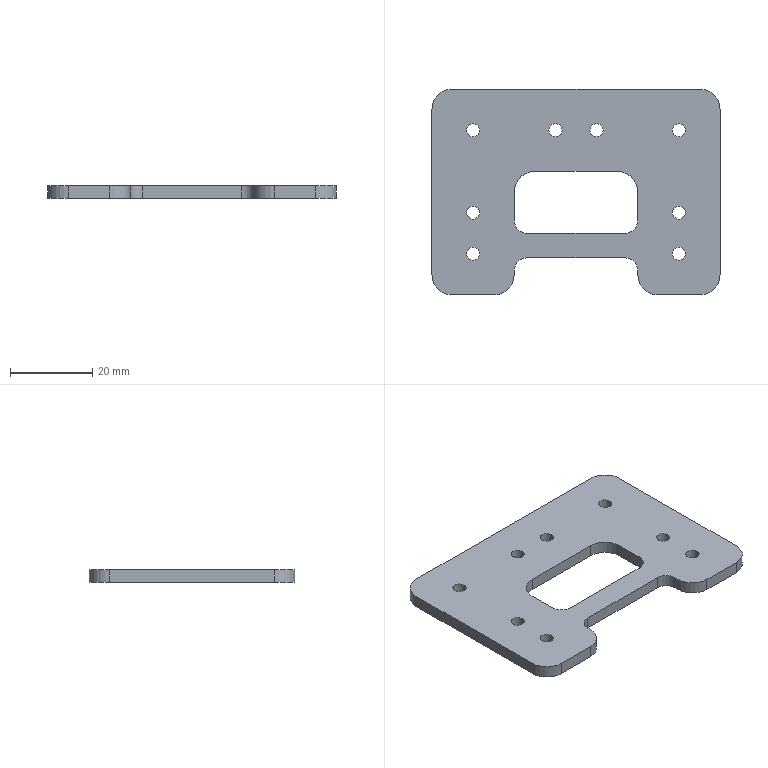Part | SolidWorks | features BaseBody 1 | 1 solid | 42 faces | box 70 x 50 x 3 mm | volume 8106 mm3 | cylinder 28 | plane 14 | commonest cylinder face diameters 3.2 x16 10 x8 6 x4
STEP:
#1=CARTESIAN_POINT('',(26.6,-15.,3.));
#2=VERTEX_POINT('',#1);
#3=CARTESIAN_POINT('',(23.4,-15.,3.));
#4=VERTEX_POINT('',#3);
#5=CARTESIAN_POINT('',(25.,-15.,3.));
#6=DIRECTION('',(0.,0.,-1.));
#7=DIRECTION('',(-1.,0.,0.));
#8=AXIS2_PLACEMENT_3D('',#5,#6,#7);
#9=CIRCLE('',#8,1.6);
#10=EDGE_CURVE('',#2,#4,#9,.T.);
#11=ORIENTED_EDGE('',*,*,#10,.F.);
#12=CARTESIAN_POINT('',(26.6,-15.,0.));
#13=VERTEX_POINT('',#12);
#14=CARTESIAN_POINT('',(26.6,-15.,3.));
#15=DIRECTION('',(0.,0.,-1.));
#16=VECTOR('',#15,1000.);
#17=LINE('',#14,#16);
#18=EDGE_CURVE('',#2,#13,#17,.T.);
#19=ORIENTED_EDGE('',*,*,#18,.T.);
#20=CARTESIAN_POINT('',(23.4,-15.,0.));
#21=VERTEX_POINT('',#20);
#22=CARTESIAN_POINT('',(25.,-15.,0.));
#23=DIRECTION('',(0.,0.,-1.));
#24=DIRECTION('',(-1.,0.,0.));
#25=AXIS2_PLACEMENT_3D('',#22,#23,#24);
#26=CIRCLE('',#25,1.6);
#27=EDGE_CURVE('',#13,#21,#26,.T.);
#28=ORIENTED_EDGE('',*,*,#27,.T.);
#29=CARTESIAN_POINT('',(23.4,-15.,3.));
#30=DIRECTION('',(0.,0.,-1.));
#31=VECTOR('',#30,1000.);
#32=LINE('',#29,#31);
#33=EDGE_CURVE('',#4,#21,#32,.T.);
#34=ORIENTED_EDGE('',*,*,#33,.F.);
#35=EDGE_LOOP('',(#11,#19,#28,#34));
#36=FACE_OUTER_BOUND('',#35,.T.);
#37=CARTESIAN_POINT('',(25.,-15.,3.));
#38=DIRECTION('',(0.,0.,-1.));
#39=DIRECTION('',(-1.,0.,0.));
#40=AXIS2_PLACEMENT_3D('',#37,#38,#39);
#41=CYLINDRICAL_SURFACE('',#40,1.6);
#42=ADVANCED_FACE('',(#36),#41,.F.);
#43=CARTESIAN_POINT('',(26.6,-5.,3.));
#44=VERTEX_POINT('',#43);
#45=CARTESIAN_POINT('',(23.4,-5.,3.));
#46=VERTEX_POINT('',#45);
#47=CARTESIAN_POINT('',(25.,-5.,3.));
#48=DIRECTION('',(0.,0.,-1.));
#49=DIRECTION('',(-1.,0.,0.));
#50=AXIS2_PLACEMENT_3D('',#47,#48,#49);
#51=CIRCLE('',#50,1.6);
#52=EDGE_CURVE('',#44,#46,#51,.T.);
#53=ORIENTED_EDGE('',*,*,#52,.F.);
#54=CARTESIAN_POINT('',(26.6,-5.,0.));
#55=VERTEX_POINT('',#54);
#56=CARTESIAN_POINT('',(26.6,-5.,3.));
#57=DIRECTION('',(0.,0.,-1.));
#58=VECTOR('',#57,1000.);
#59=LINE('',#56,#58);
#60=EDGE_CURVE('',#44,#55,#59,.T.);
#61=ORIENTED_EDGE('',*,*,#60,.T.);
#62=CARTESIAN_POINT('',(23.4,-5.,0.));
#63=VERTEX_POINT('',#62);
#64=CARTESIAN_POINT('',(25.,-5.,0.));
#65=DIRECTION('',(0.,0.,-1.));
#66=DIRECTION('',(-1.,0.,0.));
#67=AXIS2_PLACEMENT_3D('',#64,#65,#66);
#68=CIRCLE('',#67,1.6);
#69=EDGE_CURVE('',#55,#63,#68,.T.);
#70=ORIENTED_EDGE('',*,*,#69,.T.);
#71=CARTESIAN_POINT('',(23.4,-5.,3.));
#72=DIRECTION('',(0.,0.,-1.));
#73=VECTOR('',#72,1000.);
#74=LINE('',#71,#73);
#75=EDGE_CURVE('',#46,#63,#74,.T.);
#76=ORIENTED_EDGE('',*,*,#75,.F.);
#77=EDGE_LOOP('',(#53,#61,#70,#76));
#78=FACE_OUTER_BOUND('',#77,.T.);
#79=CARTESIAN_POINT('',(25.,-5.,3.));
#80=DIRECTION('',(0.,0.,-1.));
#81=DIRECTION('',(-1.,0.,0.));
#82=AXIS2_PLACEMENT_3D('',#79,#80,#81);
#83=CYLINDRICAL_SURFACE('',#82,1.6);
#84=ADVANCED_FACE('',(#78),#83,.F.);
#85=CARTESIAN_POINT('',(26.6,15.,3.));
#86=VERTEX_POINT('',#85);
#87=CARTESIAN_POINT('',(23.4,15.,3.));
#88=VERTEX_POINT('',#87);
#89=CARTESIAN_POINT('',(25.,15.,3.));
#90=DIRECTION('',(0.,0.,-1.));
#91=DIRECTION('',(-1.,0.,0.));
#92=AXIS2_PLACEMENT_3D('',#89,#90,#91);
#93=CIRCLE('',#92,1.6);
#94=EDGE_CURVE('',#86,#88,#93,.T.);
#95=ORIENTED_EDGE('',*,*,#94,.F.);
#96=CARTESIAN_POINT('',(26.6,15.,0.));
#97=VERTEX_POINT('',#96);
#98=CARTESIAN_POINT('',(26.6,15.,3.));
#99=DIRECTION('',(0.,0.,-1.));
#100=VECTOR('',#99,1000.);
#101=LINE('',#98,#100);
#102=EDGE_CURVE('',#86,#97,#101,.T.);
#103=ORIENTED_EDGE('',*,*,#102,.T.);
#104=CARTESIAN_POINT('',(23.4,15.,0.));
#105=VERTEX_POINT('',#104);
#106=CARTESIAN_POINT('',(25.,15.,0.));
#107=DIRECTION('',(0.,0.,-1.));
#108=DIRECTION('',(-1.,0.,0.));
#109=AXIS2_PLACEMENT_3D('',#106,#107,#108);
#110=CIRCLE('',#109,1.6);
#111=EDGE_CURVE('',#97,#105,#110,.T.);
#112=ORIENTED_EDGE('',*,*,#111,.T.);
#113=CARTESIAN_POINT('',(23.4,15.,3.));
#114=DIRECTION('',(0.,0.,-1.));
#115=VECTOR('',#114,1000.);
#116=LINE('',#113,#115);
#117=EDGE_CURVE('',#88,#105,#116,.T.);
#118=ORIENTED_EDGE('',*,*,#117,.F.);
#119=EDGE_LOOP('',(#95,#103,#112,#118));
#120=FACE_OUTER_BOUND('',#119,.T.);
#121=CARTESIAN_POINT('',(25.,15.,3.));
#122=DIRECTION('',(0.,0.,-1.));
#123=DIRECTION('',(-1.,0.,0.));
#124=AXIS2_PLACEMENT_3D('',#121,#122,#123);
#125=CYLINDRICAL_SURFACE('',#124,1.6);
#126=ADVANCED_FACE('',(#120),#125,.F.);
#127=CARTESIAN_POINT('',(6.6,15.,3.));
#128=VERTEX_POINT('',#127);
#129=CARTESIAN_POINT('',(3.4,15.,3.));
#130=VERTEX_POINT('',#129);
#131=CARTESIAN_POINT('',(5.,15.,3.));
#132=DIRECTION('',(0.,0.,-1.));
#133=DIRECTION('',(-1.,0.,0.));
#134=AXIS2_PLACEMENT_3D('',#131,#132,#133);
#135=CIRCLE('',#134,1.6);
#136=EDGE_CURVE('',#128,#130,#135,.T.);
#137=ORIENTED_EDGE('',*,*,#136,.F.);
#138=CARTESIAN_POINT('',(6.6,15.,0.));
#139=VERTEX_POINT('',#138);
#140=CARTESIAN_POINT('',(6.6,15.,3.));
#141=DIRECTION('',(0.,0.,-1.));
#142=VECTOR('',#141,1000.);
#143=LINE('',#140,#142);
#144=EDGE_CURVE('',#128,#139,#143,.T.);
#145=ORIENTED_EDGE('',*,*,#144,.T.);
#146=CARTESIAN_POINT('',(3.4,15.,0.));
#147=VERTEX_POINT('',#146);
#148=CARTESIAN_POINT('',(5.,15.,0.));
#149=DIRECTION('',(0.,0.,-1.));
#150=DIRECTION('',(-1.,0.,0.));
#151=AXIS2_PLACEMENT_3D('',#148,#149,#150);
#152=CIRCLE('',#151,1.6);
#153=EDGE_CURVE('',#139,#147,#152,.T.);
#154=ORIENTED_EDGE('',*,*,#153,.T.);
#155=CARTESIAN_POINT('',(3.4,15.,3.));
#156=DIRECTION('',(0.,0.,-1.));
#157=VECTOR('',#156,1000.);
#158=LINE('',#155,#157);
#159=EDGE_CURVE('',#130,#147,#158,.T.);
#160=ORIENTED_EDGE('',*,*,#159,.F.);
#161=EDGE_LOOP('',(#137,#145,#154,#160));
#162=FACE_OUTER_BOUND('',#161,.T.);
#163=CARTESIAN_POINT('',(5.,15.,3.));
#164=DIRECTION('',(0.,0.,-1.));
#165=DIRECTION('',(-1.,0.,0.));
#166=AXIS2_PLACEMENT_3D('',#163,#164,#165);
#167=CYLINDRICAL_SURFACE('',#166,1.6);
#168=ADVANCED_FACE('',(#162),#167,.F.);
#169=CARTESIAN_POINT('',(-3.4,15.,3.));
#170=VERTEX_POINT('',#169);
#171=CARTESIAN_POINT('',(-6.6,15.,3.));
#172=VERTEX_POINT('',#171);
#173=CARTESIAN_POINT('',(-5.,15.,3.));
#174=DIRECTION('',(0.,0.,-1.));
#175=DIRECTION('',(-1.,0.,0.));
#176=AXIS2_PLACEMENT_3D('',#173,#174,#175);
#177=CIRCLE('',#176,1.6);
#178=EDGE_CURVE('',#170,#172,#177,.T.);
#179=ORIENTED_EDGE('',*,*,#178,.F.);
#180=CARTESIAN_POINT('',(-3.4,15.,0.));
#181=VERTEX_POINT('',#180);
#182=CARTESIAN_POINT('',(-3.4,15.,3.));
#183=DIRECTION('',(0.,0.,-1.));
#184=VECTOR('',#183,1000.);
#185=LINE('',#182,#184);
#186=EDGE_CURVE('',#170,#181,#185,.T.);
#187=ORIENTED_EDGE('',*,*,#186,.T.);
#188=CARTESIAN_POINT('',(-6.6,15.,0.));
#189=VERTEX_POINT('',#188);
#190=CARTESIAN_POINT('',(-5.,15.,0.));
#191=DIRECTION('',(0.,0.,-1.));
#192=DIRECTION('',(-1.,0.,0.));
#193=AXIS2_PLACEMENT_3D('',#190,#191,#192);
#194=CIRCLE('',#193,1.6);
#195=EDGE_CURVE('',#181,#189,#194,.T.);
#196=ORIENTED_EDGE('',*,*,#195,.T.);
#197=CARTESIAN_POINT('',(-6.6,15.,3.));
#198=DIRECTION('',(0.,0.,-1.));
#199=VECTOR('',#198,1000.);
#200=LINE('',#197,#199);
#201=EDGE_CURVE('',#172,#189,#200,.T.);
#202=ORIENTED_EDGE('',*,*,#201,.F.);
#203=EDGE_LOOP('',(#179,#187,#196,#202));
#204=FACE_OUTER_BOUND('',#203,.T.);
#205=CARTESIAN_POINT('',(-5.,15.,3.));
#206=DIRECTION('',(0.,0.,-1.));
#207=DIRECTION('',(-1.,0.,0.));
#208=AXIS2_PLACEMENT_3D('',#205,#206,#207);
#209=CYLINDRICAL_SURFACE('',#208,1.6);
#210=ADVANCED_FACE('',(#204),#209,.F.);
#211=CARTESIAN_POINT('',(-23.4,15.,3.));
#212=VERTEX_POINT('',#211);
#213=CARTESIAN_POINT('',(-26.6,15.,3.));
#214=VERTEX_POINT('',#213);
#215=CARTESIAN_POINT('',(-25.,15.,3.));
#216=DIRECTION('',(0.,0.,-1.));
#217=DIRECTION('',(-1.,0.,0.));
#218=AXIS2_PLACEMENT_3D('',#215,#216,#217);
#219=CIRCLE('',#218,1.6);
#220=EDGE_CURVE('',#212,#214,#219,.T.);
#221=ORIENTED_EDGE('',*,*,#220,.F.);
#222=CARTESIAN_POINT('',(-23.4,15.,0.));
#223=VERTEX_POINT('',#222);
#224=CARTESIAN_POINT('',(-23.4,15.,3.));
#225=DIRECTION('',(0.,0.,-1.));
#226=VECTOR('',#225,1000.);
#227=LINE('',#224,#226);
#228=EDGE_CURVE('',#212,#223,#227,.T.);
#229=ORIENTED_EDGE('',*,*,#228,.T.);
#230=CARTESIAN_POINT('',(-26.6,15.,0.));
#231=VERTEX_POINT('',#230);
#232=CARTESIAN_POINT('',(-25.,15.,0.));
#233=DIRECTION('',(0.,0.,-1.));
#234=DIRECTION('',(-1.,0.,0.));
#235=AXIS2_PLACEMENT_3D('',#232,#233,#234);
#236=CIRCLE('',#235,1.6);
#237=EDGE_CURVE('',#223,#231,#236,.T.);
#238=ORIENTED_EDGE('',*,*,#237,.T.);
#239=CARTESIAN_POINT('',(-26.6,15.,3.));
#240=DIRECTION('',(0.,0.,-1.));
#241=VECTOR('',#240,1000.);
#242=LINE('',#239,#241);
#243=EDGE_CURVE('',#214,#231,#242,.T.);
#244=ORIENTED_EDGE('',*,*,#243,.F.);
#245=EDGE_LOOP('',(#221,#229,#238,#244));
#246=FACE_OUTER_BOUND('',#245,.T.);
#247=CARTESIAN_POINT('',(-25.,15.,3.));
#248=DIRECTION('',(0.,0.,-1.));
#249=DIRECTION('',(-1.,0.,0.));
#250=AXIS2_PLACEMENT_3D('',#247,#248,#249);
#251=CYLINDRICAL_SURFACE('',#250,1.6);
#252=ADVANCED_FACE('',(#246),#251,.F.);
#253=CARTESIAN_POINT('',(-23.4,-5.,3.));
#254=VERTEX_POINT('',#253);
#255=CARTESIAN_POINT('',(-26.6,-5.,3.));
#256=VERTEX_POINT('',#255);
#257=CARTESIAN_POINT('',(-25.,-5.,3.));
#258=DIRECTION('',(0.,0.,-1.));
#259=DIRECTION('',(-1.,0.,0.));
#260=AXIS2_PLACEMENT_3D('',#257,#258,#259);
#261=CIRCLE('',#260,1.6);
#262=EDGE_CURVE('',#254,#256,#261,.T.);
#263=ORIENTED_EDGE('',*,*,#262,.F.);
#264=CARTESIAN_POINT('',(-23.4,-5.,0.));
#265=VERTEX_POINT('',#264);
#266=CARTESIAN_POINT('',(-23.4,-5.,3.));
#267=DIRECTION('',(0.,0.,-1.));
#268=VECTOR('',#267,1000.);
#269=LINE('',#266,#268);
#270=EDGE_CURVE('',#254,#265,#269,.T.);
#271=ORIENTED_EDGE('',*,*,#270,.T.);
#272=CARTESIAN_POINT('',(-26.6,-5.,0.));
#273=VERTEX_POINT('',#272);
#274=CARTESIAN_POINT('',(-25.,-5.,0.));
#275=DIRECTION('',(0.,0.,-1.));
#276=DIRECTION('',(-1.,0.,0.));
#277=AXIS2_PLACEMENT_3D('',#274,#275,#276);
#278=CIRCLE('',#277,1.6);
#279=EDGE_CURVE('',#265,#273,#278,.T.);
#280=ORIENTED_EDGE('',*,*,#279,.T.);
#281=CARTESIAN_POINT('',(-26.6,-5.,3.));
#282=DIRECTION('',(0.,0.,-1.));
#283=VECTOR('',#282,1000.);
#284=LINE('',#281,#283);
#285=EDGE_CURVE('',#256,#273,#284,.T.);
#286=ORIENTED_EDGE('',*,*,#285,.F.);
#287=EDGE_LOOP('',(#263,#271,#280,#286));
#288=FACE_OUTER_BOUND('',#287,.T.);
#289=CARTESIAN_POINT('',(-25.,-5.,3.));
#290=DIRECTION('',(0.,0.,-1.));
#291=DIRECTION('',(-1.,0.,0.));
#292=AXIS2_PLACEMENT_3D('',#289,#290,#291);
#293=CYLINDRICAL_SURFACE('',#292,1.6);
#294=ADVANCED_FACE('',(#288),#293,.F.);
#295=CARTESIAN_POINT('',(-23.4,-15.,3.));
#296=VERTEX_POINT('',#295);
#297=CARTESIAN_POINT('',(-26.6,-15.,3.));
#298=VERTEX_POINT('',#297);
#299=CARTESIAN_POINT('',(-25.,-15.,3.));
#300=DIRECTION('',(0.,0.,-1.));
#301=DIRECTION('',(-1.,0.,0.));
#302=AXIS2_PLACEMENT_3D('',#299,#300,#301);
#303=CIRCLE('',#302,1.6);
#304=EDGE_CURVE('',#296,#298,#303,.T.);
#305=ORIENTED_EDGE('',*,*,#304,.F.);
#306=CARTESIAN_POINT('',(-23.4,-15.,0.));
#307=VERTEX_POINT('',#306);
#308=CARTESIAN_POINT('',(-23.4,-15.,3.));
#309=DIRECTION('',(0.,0.,-1.));
#310=VECTOR('',#309,1000.);
#311=LINE('',#308,#310);
#312=EDGE_CURVE('',#296,#307,#311,.T.);
#313=ORIENTED_EDGE('',*,*,#312,.T.);
#314=CARTESIAN_POINT('',(-26.6,-15.,0.));
#315=VERTEX_POINT('',#314);
#316=CARTESIAN_POINT('',(-25.,-15.,0.));
#317=DIRECTION('',(0.,0.,-1.));
#318=DIRECTION('',(-1.,0.,0.));
#319=AXIS2_PLACEMENT_3D('',#316,#317,#318);
#320=CIRCLE('',#319,1.6);
#321=EDGE_CURVE('',#307,#315,#320,.T.);
#322=ORIENTED_EDGE('',*,*,#321,.T.);
#323=CARTESIAN_POINT('',(-26.6,-15.,3.));
#324=DIRECTION('',(0.,0.,-1.));
#325=VECTOR('',#324,1000.);
#326=LINE('',#323,#325);
#327=EDGE_CURVE('',#298,#315,#326,.T.);
#328=ORIENTED_EDGE('',*,*,#327,.F.);
#329=EDGE_LOOP('',(#305,#313,#322,#328));
#330=FACE_OUTER_BOUND('',#329,.T.);
#331=CARTESIAN_POINT('',(-25.,-15.,3.));
#332=DIRECTION('',(0.,0.,-1.));
#333=DIRECTION('',(-1.,0.,0.));
#334=AXIS2_PLACEMENT_3D('',#331,#332,#333);
#335=CYLINDRICAL_SURFACE('',#334,1.6);
#336=ADVANCED_FACE('',(#330),#335,.F.);
#337=CARTESIAN_POINT('',(25.,-15.,0.));
#338=DIRECTION('',(0.,0.,-1.));
#339=DIRECTION('',(-1.,0.,0.));
#340=AXIS2_PLACEMENT_3D('',#337,#338,#339);
#341=CIRCLE('',#340,1.6);
#342=EDGE_CURVE('',#21,#13,#341,.T.);
#343=ORIENTED_EDGE('',*,*,#342,.F.);
#344=ORIENTED_EDGE('',*,*,#27,.F.);
#345=EDGE_LOOP('',(#343,#344));
#346=FACE_BOUND('',#345,.T.);
#347=CARTESIAN_POINT('',(25.,-5.,0.));
#348=DIRECTION('',(0.,0.,-1.));
#349=DIRECTION('',(-1.,0.,0.));
#350=AXIS2_PLACEMENT_3D('',#347,#348,#349);
#351=CIRCLE('',#350,1.6);
#352=EDGE_CURVE('',#63,#55,#351,.T.);
#353=ORIENTED_EDGE('',*,*,#352,.F.);
#354=ORIENTED_EDGE('',*,*,#69,.F.);
#355=EDGE_LOOP('',(#353,#354));
#356=FACE_BOUND('',#355,.T.);
#357=CARTESIAN_POINT('',(25.,15.,0.));
#358=DIRECTION('',(0.,0.,-1.));
#359=DIRECTION('',(-1.,0.,0.));
#360=AXIS2_PLACEMENT_3D('',#357,#358,#359);
#361=CIRCLE('',#360,1.6);
#362=EDGE_CURVE('',#105,#97,#361,.T.);
#363=ORIENTED_EDGE('',*,*,#362,.F.);
#364=ORIENTED_EDGE('',*,*,#111,.F.);
#365=EDGE_LOOP('',(#363,#364));
#366=FACE_BOUND('',#365,.T.);
#367=CARTESIAN_POINT('',(5.,15.,0.));
#368=DIRECTION('',(0.,0.,-1.));
#369=DIRECTION('',(-1.,0.,0.));
#370=AXIS2_PLACEMENT_3D('',#367,#368,#369);
#371=CIRCLE('',#370,1.6);
#372=EDGE_CURVE('',#147,#139,#371,.T.);
#373=ORIENTED_EDGE('',*,*,#372,.F.);
#374=ORIENTED_EDGE('',*,*,#153,.F.);
#375=EDGE_LOOP('',(#373,#374));
#376=FACE_BOUND('',#375,.T.);
#377=CARTESIAN_POINT('',(-5.,15.,0.));
#378=DIRECTION('',(0.,0.,-1.));
#379=DIRECTION('',(-1.,0.,0.));
#380=AXIS2_PLACEMENT_3D('',#377,#378,#379);
#381=CIRCLE('',#380,1.6);
#382=EDGE_CURVE('',#189,#181,#381,.T.);
#383=ORIENTED_EDGE('',*,*,#382,.F.);
#384=ORIENTED_EDGE('',*,*,#195,.F.);
#385=EDGE_LOOP('',(#383,#384));
#386=FACE_BOUND('',#385,.T.);
#387=CARTESIAN_POINT('',(-25.,15.,0.));
#388=DIRECTION('',(0.,0.,-1.));
#389=DIRECTION('',(-1.,0.,0.));
#390=AXIS2_PLACEMENT_3D('',#387,#388,#389);
#391=CIRCLE('',#390,1.6);
#392=EDGE_CURVE('',#231,#223,#391,.T.);
#393=ORIENTED_EDGE('',*,*,#392,.F.);
#394=ORIENTED_EDGE('',*,*,#237,.F.);
#395=EDGE_LOOP('',(#393,#394));
#396=FACE_BOUND('',#395,.T.);
#397=CARTESIAN_POINT('',(-25.,-5.,0.));
#398=DIRECTION('',(0.,0.,-1.));
#399=DIRECTION('',(-1.,0.,0.));
#400=AXIS2_PLACEMENT_3D('',#397,#398,#399);
#401=CIRCLE('',#400,1.6);
#402=EDGE_CURVE('',#273,#265,#401,.T.);
#403=ORIENTED_EDGE('',*,*,#402,.F.);
#404=ORIENTED_EDGE('',*,*,#279,.F.);
#405=EDGE_LOOP('',(#403,#404));
#406=FACE_BOUND('',#405,.T.);
#407=CARTESIAN_POINT('',(-25.,-15.,0.));
#408=DIRECTION('',(0.,0.,-1.));
#409=DIRECTION('',(-1.,0.,0.));
#410=AXIS2_PLACEMENT_3D('',#407,#408,#409);
#411=CIRCLE('',#410,1.6);
#412=EDGE_CURVE('',#315,#307,#411,.T.);
#413=ORIENTED_EDGE('',*,*,#412,.F.);
#414=ORIENTED_EDGE('',*,*,#321,.F.);
#415=EDGE_LOOP('',(#413,#414));
#416=FACE_BOUND('',#415,.T.);
#417=CARTESIAN_POINT('',(-12.,-10.,0.));
#418=VERTEX_POINT('',#417);
#419=CARTESIAN_POINT('',(-15.,-7.,0.));
#420=VERTEX_POINT('',#419);
#421=CARTESIAN_POINT('',(-12.,-7.,0.));
#422=DIRECTION('',(0.,0.,-1.));
#423=DIRECTION('',(1.,0.,0.));
#424=AXIS2_PLACEMENT_3D('',#421,#422,#423);
#425=CIRCLE('',#424,3.);
#426=EDGE_CURVE('',#418,#420,#425,.T.);
#427=ORIENTED_EDGE('',*,*,#426,.F.);
#428=CARTESIAN_POINT('',(12.,-10.,0.));
#429=VERTEX_POINT('',#428);
#430=CARTESIAN_POINT('',(0.,-10.,0.));
#431=DIRECTION('',(-1.,0.,0.));
#432=VECTOR('',#431,1000.);
#433=LINE('',#430,#432);
#434=EDGE_CURVE('',#429,#418,#433,.T.);
#435=ORIENTED_EDGE('',*,*,#434,.F.);
#436=CARTESIAN_POINT('',(15.,-7.,0.));
#437=VERTEX_POINT('',#436);
#438=CARTESIAN_POINT('',(12.,-7.,0.));
#439=DIRECTION('',(0.,0.,-1.));
#440=DIRECTION('',(1.,0.,0.));
#441=AXIS2_PLACEMENT_3D('',#438,#439,#440);
#442=CIRCLE('',#441,3.);
#443=EDGE_CURVE('',#437,#429,#442,.T.);
#444=ORIENTED_EDGE('',*,*,#443,.F.);
#445=CARTESIAN_POINT('',(15.,0.,0.));
#446=VERTEX_POINT('',#445);
#447=CARTESIAN_POINT('',(15.,0.,0.));
#448=DIRECTION('',(0.,-1.,0.));
#449=VECTOR('',#448,1000.);
#450=LINE('',#447,#449);
#451=EDGE_CURVE('',#446,#437,#450,.T.);
#452=ORIENTED_EDGE('',*,*,#451,.F.);
#453=CARTESIAN_POINT('',(10.,5.,0.));
#454=VERTEX_POINT('',#453);
#455=CARTESIAN_POINT('',(10.,0.,0.));
#456=DIRECTION('',(0.,0.,-1.));
#457=DIRECTION('',(-1.,0.,0.));
#458=AXIS2_PLACEMENT_3D('',#455,#456,#457);
#459=CIRCLE('',#458,5.);
#460=EDGE_CURVE('',#454,#446,#459,.T.);
#461=ORIENTED_EDGE('',*,*,#460,.F.);
#462=CARTESIAN_POINT('',(-10.,5.,0.));
#463=VERTEX_POINT('',#462);
#464=CARTESIAN_POINT('',(0.,5.,0.));
#465=DIRECTION('',(1.,0.,0.));
#466=VECTOR('',#465,1000.);
#467=LINE('',#464,#466);
#468=EDGE_CURVE('',#463,#454,#467,.T.);
#469=ORIENTED_EDGE('',*,*,#468,.F.);
#470=CARTESIAN_POINT('',(-15.,0.,0.));
#471=VERTEX_POINT('',#470);
#472=CARTESIAN_POINT('',(-10.,0.,0.));
#473=DIRECTION('',(0.,0.,-1.));
#474=DIRECTION('',(-1.,0.,0.));
#475=AXIS2_PLACEMENT_3D('',#472,#473,#474);
#476=CIRCLE('',#475,5.);
#477=EDGE_CURVE('',#471,#463,#476,.T.);
#478=ORIENTED_EDGE('',*,*,#477,.F.);
#479=CARTESIAN_POINT('',(-15.,0.,0.));
#480=DIRECTION('',(0.,1.,0.));
#481=VECTOR('',#480,1000.);
#482=LINE('',#479,#481);
#483=EDGE_CURVE('',#420,#471,#482,.T.);
#484=ORIENTED_EDGE('',*,*,#483,.F.);
#485=EDGE_LOOP('',(#427,#435,#444,#452,#461,#469,#478,#484));
#486=FACE_BOUND('',#485,.T.);
#487=CARTESIAN_POINT('',(-15.,-19.,0.));
#488=VERTEX_POINT('',#487);
#489=CARTESIAN_POINT('',(-12.,-16.,0.));
#490=VERTEX_POINT('',#489);
#491=CARTESIAN_POINT('',(-12.,-19.,0.));
#492=DIRECTION('',(0.,0.,-1.));
#493=DIRECTION('',(1.,0.,0.));
#494=AXIS2_PLACEMENT_3D('',#491,#492,#493);
#495=CIRCLE('',#494,3.);
#496=EDGE_CURVE('',#488,#490,#495,.T.);
#497=ORIENTED_EDGE('',*,*,#496,.F.);
#498=CARTESIAN_POINT('',(-15.,-20.,0.));
#499=VERTEX_POINT('',#498);
#500=CARTESIAN_POINT('',(-15.,-25.,0.));
#501=DIRECTION('',(0.,-1.,0.));
#502=VECTOR('',#501,1000.);
#503=LINE('',#500,#502);
#504=EDGE_CURVE('',#488,#499,#503,.T.);
#505=ORIENTED_EDGE('',*,*,#504,.T.);
#506=CARTESIAN_POINT('',(-20.,-25.,0.));
#507=VERTEX_POINT('',#506);
#508=CARTESIAN_POINT('',(-20.,-20.,0.));
#509=DIRECTION('',(0.,0.,1.));
#510=DIRECTION('',(1.,0.,0.));
#511=AXIS2_PLACEMENT_3D('',#508,#509,#510);
#512=CIRCLE('',#511,5.);
#513=EDGE_CURVE('',#507,#499,#512,.T.);
#514=ORIENTED_EDGE('',*,*,#513,.F.);
#515=CARTESIAN_POINT('',(-30.,-25.,0.));
#516=VERTEX_POINT('',#515);
#517=CARTESIAN_POINT('',(0.,-25.,0.));
#518=DIRECTION('',(1.,0.,0.));
#519=VECTOR('',#518,1000.);
#520=LINE('',#517,#519);
#521=EDGE_CURVE('',#516,#507,#520,.T.);
#522=ORIENTED_EDGE('',*,*,#521,.F.);
#523=CARTESIAN_POINT('',(-35.,-20.,0.));
#524=VERTEX_POINT('',#523);
#525=CARTESIAN_POINT('',(-30.,-20.,0.));
#526=DIRECTION('',(0.,0.,1.));
#527=DIRECTION('',(-1.,0.,0.));
#528=AXIS2_PLACEMENT_3D('',#525,#526,#527);
#529=CIRCLE('',#528,5.);
#530=EDGE_CURVE('',#524,#516,#529,.T.);
#531=ORIENTED_EDGE('',*,*,#530,.F.);
#532=CARTESIAN_POINT('',(-35.,20.,0.));
#533=VERTEX_POINT('',#532);
#534=CARTESIAN_POINT('',(-35.,0.,0.));
#535=DIRECTION('',(0.,-1.,0.));
#536=VECTOR('',#535,1000.);
#537=LINE('',#534,#536);
#538=EDGE_CURVE('',#533,#524,#537,.T.);
#539=ORIENTED_EDGE('',*,*,#538,.F.);
#540=CARTESIAN_POINT('',(-30.,25.,0.));
#541=VERTEX_POINT('',#540);
#542=CARTESIAN_POINT('',(-30.,20.,0.));
#543=DIRECTION('',(0.,0.,1.));
#544=DIRECTION('',(-1.,0.,0.));
#545=AXIS2_PLACEMENT_3D('',#542,#543,#544);
#546=CIRCLE('',#545,5.);
#547=EDGE_CURVE('',#541,#533,#546,.T.);
#548=ORIENTED_EDGE('',*,*,#547,.F.);
#549=CARTESIAN_POINT('',(30.,25.,0.));
#550=VERTEX_POINT('',#549);
#551=CARTESIAN_POINT('',(0.,25.,0.));
#552=DIRECTION('',(-1.,0.,0.));
#553=VECTOR('',#552,1000.);
#554=LINE('',#551,#553);
#555=EDGE_CURVE('',#550,#541,#554,.T.);
#556=ORIENTED_EDGE('',*,*,#555,.F.);
#557=CARTESIAN_POINT('',(35.,20.,0.));
#558=VERTEX_POINT('',#557);
#559=CARTESIAN_POINT('',(30.,20.,0.));
#560=DIRECTION('',(0.,0.,1.));
#561=DIRECTION('',(-1.,0.,0.));
#562=AXIS2_PLACEMENT_3D('',#559,#560,#561);
#563=CIRCLE('',#562,5.);
#564=EDGE_CURVE('',#558,#550,#563,.T.);
#565=ORIENTED_EDGE('',*,*,#564,.F.);
#566=CARTESIAN_POINT('',(35.,-20.,0.));
#567=VERTEX_POINT('',#566);
#568=CARTESIAN_POINT('',(35.,0.,0.));
#569=DIRECTION('',(0.,1.,0.));
#570=VECTOR('',#569,1000.);
#571=LINE('',#568,#570);
#572=EDGE_CURVE('',#567,#558,#571,.T.);
#573=ORIENTED_EDGE('',*,*,#572,.F.);
#574=CARTESIAN_POINT('',(30.,-25.,0.));
#575=VERTEX_POINT('',#574);
#576=CARTESIAN_POINT('',(30.,-20.,0.));
#577=DIRECTION('',(0.,0.,1.));
#578=DIRECTION('',(-1.,0.,0.));
#579=AXIS2_PLACEMENT_3D('',#576,#577,#578);
#580=CIRCLE('',#579,5.);
#581=EDGE_CURVE('',#575,#567,#580,.T.);
#582=ORIENTED_EDGE('',*,*,#581,.F.);
#583=CARTESIAN_POINT('',(20.,-25.,0.));
#584=VERTEX_POINT('',#583);
#585=CARTESIAN_POINT('',(0.,-25.,0.));
#586=DIRECTION('',(1.,0.,0.));
#587=VECTOR('',#586,1000.);
#588=LINE('',#585,#587);
#589=EDGE_CURVE('',#584,#575,#588,.T.);
#590=ORIENTED_EDGE('',*,*,#589,.F.);
#591=CARTESIAN_POINT('',(15.,-20.,0.));
#592=VERTEX_POINT('',#591);
#593=CARTESIAN_POINT('',(20.,-20.,0.));
#594=DIRECTION('',(0.,0.,1.));
#595=DIRECTION('',(1.,0.,0.));
#596=AXIS2_PLACEMENT_3D('',#593,#594,#595);
#597=CIRCLE('',#596,5.);
#598=EDGE_CURVE('',#592,#584,#597,.T.);
#599=ORIENTED_EDGE('',*,*,#598,.F.);
#600=CARTESIAN_POINT('',(15.,-19.,0.));
#601=VERTEX_POINT('',#600);
#602=CARTESIAN_POINT('',(15.,5.,0.));
#603=DIRECTION('',(0.,1.,0.));
#604=VECTOR('',#603,1000.);
#605=LINE('',#602,#604);
#606=EDGE_CURVE('',#592,#601,#605,.T.);
#607=ORIENTED_EDGE('',*,*,#606,.T.);
#608=CARTESIAN_POINT('',(12.,-16.,0.));
#609=VERTEX_POINT('',#608);
#610=CARTESIAN_POINT('',(12.,-19.,0.));
#611=DIRECTION('',(0.,0.,-1.));
#612=DIRECTION('',(1.,0.,0.));
#613=AXIS2_PLACEMENT_3D('',#610,#611,#612);
#614=CIRCLE('',#613,3.);
#615=EDGE_CURVE('',#609,#601,#614,.T.);
#616=ORIENTED_EDGE('',*,*,#615,.F.);
#617=CARTESIAN_POINT('',(0.,-16.,0.));
#618=DIRECTION('',(1.,0.,0.));
#619=VECTOR('',#618,1000.);
#620=LINE('',#617,#619);
#621=EDGE_CURVE('',#490,#609,#620,.T.);
#622=ORIENTED_EDGE('',*,*,#621,.F.);
#623=EDGE_LOOP('',(#497,#505,#514,#522,#531,#539,#548,#556,#565,#573,#582,#590,#599,#607,#616,#622));
#624=FACE_OUTER_BOUND('',#623,.T.);
#625=CARTESIAN_POINT('',(0.,0.,0.));
#626=DIRECTION('',(0.,0.,1.));
#627=DIRECTION('',(1.,0.,0.));
#628=AXIS2_PLACEMENT_3D('',#625,#626,#627);
#629=PLANE('',#628);
#630=ADVANCED_FACE('',(#346,#356,#366,#376,#386,#396,#406,#416,#486,#624),#629,.F.);
#631=ORIENTED_EDGE('',*,*,#18,.F.);
#632=CARTESIAN_POINT('',(25.,-15.,3.));
#633=DIRECTION('',(0.,0.,-1.));
#634=DIRECTION('',(-1.,0.,0.));
#635=AXIS2_PLACEMENT_3D('',#632,#633,#634);
#636=CIRCLE('',#635,1.6);
#637=EDGE_CURVE('',#4,#2,#636,.T.);
#638=ORIENTED_EDGE('',*,*,#637,.F.);
#639=ORIENTED_EDGE('',*,*,#33,.T.);
#640=ORIENTED_EDGE('',*,*,#342,.T.);
#641=EDGE_LOOP('',(#631,#638,#639,#640));
#642=FACE_OUTER_BOUND('',#641,.T.);
#643=CARTESIAN_POINT('',(25.,-15.,3.));
#644=DIRECTION('',(0.,0.,-1.));
#645=DIRECTION('',(-1.,0.,0.));
#646=AXIS2_PLACEMENT_3D('',#643,#644,#645);
#647=CYLINDRICAL_SURFACE('',#646,1.6);
#648=ADVANCED_FACE('',(#642),#647,.F.);
#649=ORIENTED_EDGE('',*,*,#60,.F.);
#650=CARTESIAN_POINT('',(25.,-5.,3.));
#651=DIRECTION('',(0.,0.,-1.));
#652=DIRECTION('',(-1.,0.,0.));
#653=AXIS2_PLACEMENT_3D('',#650,#651,#652);
#654=CIRCLE('',#653,1.6);
#655=EDGE_CURVE('',#46,#44,#654,.T.);
#656=ORIENTED_EDGE('',*,*,#655,.F.);
#657=ORIENTED_EDGE('',*,*,#75,.T.);
#658=ORIENTED_EDGE('',*,*,#352,.T.);
#659=EDGE_LOOP('',(#649,#656,#657,#658));
#660=FACE_OUTER_BOUND('',#659,.T.);
#661=CARTESIAN_POINT('',(25.,-5.,3.));
#662=DIRECTION('',(0.,0.,-1.));
#663=DIRECTION('',(-1.,0.,0.));
#664=AXIS2_PLACEMENT_3D('',#661,#662,#663);
#665=CYLINDRICAL_SURFACE('',#664,1.6);
#666=ADVANCED_FACE('',(#660),#665,.F.);
#667=ORIENTED_EDGE('',*,*,#102,.F.);
#668=CARTESIAN_POINT('',(25.,15.,3.));
#669=DIRECTION('',(0.,0.,-1.));
#670=DIRECTION('',(-1.,0.,0.));
#671=AXIS2_PLACEMENT_3D('',#668,#669,#670);
#672=CIRCLE('',#671,1.6);
#673=EDGE_CURVE('',#88,#86,#672,.T.);
#674=ORIENTED_EDGE('',*,*,#673,.F.);
#675=ORIENTED_EDGE('',*,*,#117,.T.);
#676=ORIENTED_EDGE('',*,*,#362,.T.);
#677=EDGE_LOOP('',(#667,#674,#675,#676));
#678=FACE_OUTER_BOUND('',#677,.T.);
#679=CARTESIAN_POINT('',(25.,15.,3.));
#680=DIRECTION('',(0.,0.,-1.));
#681=DIRECTION('',(-1.,0.,0.));
#682=AXIS2_PLACEMENT_3D('',#679,#680,#681);
#683=CYLINDRICAL_SURFACE('',#682,1.6);
#684=ADVANCED_FACE('',(#678),#683,.F.);
#685=ORIENTED_EDGE('',*,*,#144,.F.);
#686=CARTESIAN_POINT('',(5.,15.,3.));
#687=DIRECTION('',(0.,0.,-1.));
#688=DIRECTION('',(-1.,0.,0.));
#689=AXIS2_PLACEMENT_3D('',#686,#687,#688);
#690=CIRCLE('',#689,1.6);
#691=EDGE_CURVE('',#130,#128,#690,.T.);
#692=ORIENTED_EDGE('',*,*,#691,.F.);
#693=ORIENTED_EDGE('',*,*,#159,.T.);
#694=ORIENTED_EDGE('',*,*,#372,.T.);
#695=EDGE_LOOP('',(#685,#692,#693,#694));
#696=FACE_OUTER_BOUND('',#695,.T.);
#697=CARTESIAN_POINT('',(5.,15.,3.));
#698=DIRECTION('',(0.,0.,-1.));
#699=DIRECTION('',(-1.,0.,0.));
#700=AXIS2_PLACEMENT_3D('',#697,#698,#699);
#701=CYLINDRICAL_SURFACE('',#700,1.6);
#702=ADVANCED_FACE('',(#696),#701,.F.);
#703=ORIENTED_EDGE('',*,*,#186,.F.);
#704=CARTESIAN_POINT('',(-5.,15.,3.));
#705=DIRECTION('',(0.,0.,-1.));
#706=DIRECTION('',(-1.,0.,0.));
#707=AXIS2_PLACEMENT_3D('',#704,#705,#706);
#708=CIRCLE('',#707,1.6);
#709=EDGE_CURVE('',#172,#170,#708,.T.);
#710=ORIENTED_EDGE('',*,*,#709,.F.);
#711=ORIENTED_EDGE('',*,*,#201,.T.);
#712=ORIENTED_EDGE('',*,*,#382,.T.);
#713=EDGE_LOOP('',(#703,#710,#711,#712));
#714=FACE_OUTER_BOUND('',#713,.T.);
#715=CARTESIAN_POINT('',(-5.,15.,3.));
#716=DIRECTION('',(0.,0.,-1.));
#717=DIRECTION('',(-1.,0.,0.));
#718=AXIS2_PLACEMENT_3D('',#715,#716,#717);
#719=CYLINDRICAL_SURFACE('',#718,1.6);
#720=ADVANCED_FACE('',(#714),#719,.F.);
#721=ORIENTED_EDGE('',*,*,#228,.F.);
#722=CARTESIAN_POINT('',(-25.,15.,3.));
#723=DIRECTION('',(0.,0.,-1.));
#724=DIRECTION('',(-1.,0.,0.));
#725=AXIS2_PLACEMENT_3D('',#722,#723,#724);
#726=CIRCLE('',#725,1.6);
#727=EDGE_CURVE('',#214,#212,#726,.T.);
#728=ORIENTED_EDGE('',*,*,#727,.F.);
#729=ORIENTED_EDGE('',*,*,#243,.T.);
#730=ORIENTED_EDGE('',*,*,#392,.T.);
#731=EDGE_LOOP('',(#721,#728,#729,#730));
#732=FACE_OUTER_BOUND('',#731,.T.);
#733=CARTESIAN_POINT('',(-25.,15.,3.));
#734=DIRECTION('',(0.,0.,-1.));
#735=DIRECTION('',(-1.,0.,0.));
#736=AXIS2_PLACEMENT_3D('',#733,#734,#735);
#737=CYLINDRICAL_SURFACE('',#736,1.6);
#738=ADVANCED_FACE('',(#732),#737,.F.);
#739=ORIENTED_EDGE('',*,*,#270,.F.);
#740=CARTESIAN_POINT('',(-25.,-5.,3.));
#741=DIRECTION('',(0.,0.,-1.));
#742=DIRECTION('',(-1.,0.,0.));
#743=AXIS2_PLACEMENT_3D('',#740,#741,#742);
#744=CIRCLE('',#743,1.6);
#745=EDGE_CURVE('',#256,#254,#744,.T.);
#746=ORIENTED_EDGE('',*,*,#745,.F.);
#747=ORIENTED_EDGE('',*,*,#285,.T.);
#748=ORIENTED_EDGE('',*,*,#402,.T.);
#749=EDGE_LOOP('',(#739,#746,#747,#748));
#750=FACE_OUTER_BOUND('',#749,.T.);
#751=CARTESIAN_POINT('',(-25.,-5.,3.));
#752=DIRECTION('',(0.,0.,-1.));
#753=DIRECTION('',(-1.,0.,0.));
#754=AXIS2_PLACEMENT_3D('',#751,#752,#753);
#755=CYLINDRICAL_SURFACE('',#754,1.6);
#756=ADVANCED_FACE('',(#750),#755,.F.);
#757=ORIENTED_EDGE('',*,*,#312,.F.);
#758=CARTESIAN_POINT('',(-25.,-15.,3.));
#759=DIRECTION('',(0.,0.,-1.));
#760=DIRECTION('',(-1.,0.,0.));
#761=AXIS2_PLACEMENT_3D('',#758,#759,#760);
#762=CIRCLE('',#761,1.6);
#763=EDGE_CURVE('',#298,#296,#762,.T.);
#764=ORIENTED_EDGE('',*,*,#763,.F.);
#765=ORIENTED_EDGE('',*,*,#327,.T.);
#766=ORIENTED_EDGE('',*,*,#412,.T.);
#767=EDGE_LOOP('',(#757,#764,#765,#766));
#768=FACE_OUTER_BOUND('',#767,.T.);
#769=CARTESIAN_POINT('',(-25.,-15.,3.));
#770=DIRECTION('',(0.,0.,-1.));
#771=DIRECTION('',(-1.,0.,0.));
#772=AXIS2_PLACEMENT_3D('',#769,#770,#771);
#773=CYLINDRICAL_SURFACE('',#772,1.6);
#774=ADVANCED_FACE('',(#768),#773,.F.);
#775=CARTESIAN_POINT('',(-15.,-7.,3.));
#776=VERTEX_POINT('',#775);
#777=CARTESIAN_POINT('',(-15.,-7.,0.));
#778=DIRECTION('',(0.,0.,1.));
#779=VECTOR('',#778,1000.);
#780=LINE('',#777,#779);
#781=EDGE_CURVE('',#420,#776,#780,.T.);
#782=ORIENTED_EDGE('',*,*,#781,.F.);
#783=ORIENTED_EDGE('',*,*,#483,.T.);
#784=CARTESIAN_POINT('',(-15.,0.,3.));
#785=VERTEX_POINT('',#784);
#786=CARTESIAN_POINT('',(-15.,0.,0.));
#787=DIRECTION('',(0.,0.,-1.));
#788=VECTOR('',#787,1000.);
#789=LINE('',#786,#788);
#790=EDGE_CURVE('',#785,#471,#789,.T.);
#791=ORIENTED_EDGE('',*,*,#790,.F.);
#792=CARTESIAN_POINT('',(-15.,-25.,3.));
#793=DIRECTION('',(0.,1.,0.));
#794=VECTOR('',#793,1000.);
#795=LINE('',#792,#794);
#796=EDGE_CURVE('',#776,#785,#795,.T.);
#797=ORIENTED_EDGE('',*,*,#796,.F.);
#798=EDGE_LOOP('',(#782,#783,#791,#797));
#799=FACE_OUTER_BOUND('',#798,.T.);
#800=CARTESIAN_POINT('',(-15.,-25.,0.));
#801=DIRECTION('',(-1.,0.,0.));
#802=DIRECTION('',(0.,-1.,0.));
#803=AXIS2_PLACEMENT_3D('',#800,#801,#802);
#804=PLANE('',#803);
#805=ADVANCED_FACE('',(#799),#804,.F.);
#806=ORIENTED_EDGE('',*,*,#781,.T.);
#807=CARTESIAN_POINT('',(-12.,-10.,3.));
#808=VERTEX_POINT('',#807);
#809=CARTESIAN_POINT('',(-12.,-7.,3.));
#810=DIRECTION('',(0.,0.,-1.));
#811=DIRECTION('',(1.,0.,0.));
#812=AXIS2_PLACEMENT_3D('',#809,#810,#811);
#813=CIRCLE('',#812,3.);
#814=EDGE_CURVE('',#808,#776,#813,.T.);
#815=ORIENTED_EDGE('',*,*,#814,.F.);
#816=CARTESIAN_POINT('',(-12.,-10.,0.));
#817=DIRECTION('',(0.,0.,1.));
#818=VECTOR('',#817,1000.);
#819=LINE('',#816,#818);
#820=EDGE_CURVE('',#418,#808,#819,.T.);
#821=ORIENTED_EDGE('',*,*,#820,.F.);
#822=ORIENTED_EDGE('',*,*,#426,.T.);
#823=EDGE_LOOP('',(#806,#815,#821,#822));
#824=FACE_OUTER_BOUND('',#823,.T.);
#825=CARTESIAN_POINT('',(-12.,-7.,0.));
#826=DIRECTION('',(0.,0.,1.));
#827=DIRECTION('',(1.,0.,0.));
#828=AXIS2_PLACEMENT_3D('',#825,#826,#827);
#829=CYLINDRICAL_SURFACE('',#828,3.);
#830=ADVANCED_FACE('',(#824),#829,.F.);
#831=ORIENTED_EDGE('',*,*,#434,.T.);
#832=ORIENTED_EDGE('',*,*,#820,.T.);
#833=CARTESIAN_POINT('',(12.,-10.,3.));
#834=VERTEX_POINT('',#833);
#835=CARTESIAN_POINT('',(15.,-10.,3.));
#836=DIRECTION('',(1.,0.,0.));
#837=VECTOR('',#836,1000.);
#838=LINE('',#835,#837);
#839=EDGE_CURVE('',#808,#834,#838,.T.);
#840=ORIENTED_EDGE('',*,*,#839,.T.);
#841=CARTESIAN_POINT('',(12.,-10.,0.));
#842=DIRECTION('',(0.,0.,-1.));
#843=VECTOR('',#842,1000.);
#844=LINE('',#841,#843);
#845=EDGE_CURVE('',#834,#429,#844,.T.);
#846=ORIENTED_EDGE('',*,*,#845,.T.);
#847=EDGE_LOOP('',(#831,#832,#840,#846));
#848=FACE_OUTER_BOUND('',#847,.T.);
#849=CARTESIAN_POINT('',(15.,-10.,0.));
#850=DIRECTION('',(0.,1.,0.));
#851=DIRECTION('',(-1.,0.,0.));
#852=AXIS2_PLACEMENT_3D('',#849,#850,#851);
#853=PLANE('',#852);
#854=ADVANCED_FACE('',(#848),#853,.T.);
#855=ORIENTED_EDGE('',*,*,#845,.F.);
#856=CARTESIAN_POINT('',(15.,-7.,3.));
#857=VERTEX_POINT('',#856);
#858=CARTESIAN_POINT('',(12.,-7.,3.));
#859=DIRECTION('',(0.,0.,-1.));
#860=DIRECTION('',(1.,0.,0.));
#861=AXIS2_PLACEMENT_3D('',#858,#859,#860);
#862=CIRCLE('',#861,3.);
#863=EDGE_CURVE('',#857,#834,#862,.T.);
#864=ORIENTED_EDGE('',*,*,#863,.F.);
#865=CARTESIAN_POINT('',(15.,-7.,0.));
#866=DIRECTION('',(0.,0.,1.));
#867=VECTOR('',#866,1000.);
#868=LINE('',#865,#867);
#869=EDGE_CURVE('',#437,#857,#868,.T.);
#870=ORIENTED_EDGE('',*,*,#869,.F.);
#871=ORIENTED_EDGE('',*,*,#443,.T.);
#872=EDGE_LOOP('',(#855,#864,#870,#871));
#873=FACE_OUTER_BOUND('',#872,.T.);
#874=CARTESIAN_POINT('',(12.,-7.,0.));
#875=DIRECTION('',(0.,0.,1.));
#876=DIRECTION('',(1.,0.,0.));
#877=AXIS2_PLACEMENT_3D('',#874,#875,#876);
#878=CYLINDRICAL_SURFACE('',#877,3.);
#879=ADVANCED_FACE('',(#873),#878,.F.);
#880=ORIENTED_EDGE('',*,*,#869,.T.);
#881=CARTESIAN_POINT('',(15.,0.,3.));
#882=VERTEX_POINT('',#881);
#883=CARTESIAN_POINT('',(15.,5.,3.));
#884=DIRECTION('',(0.,-1.,0.));
#885=VECTOR('',#884,1000.);
#886=LINE('',#883,#885);
#887=EDGE_CURVE('',#882,#857,#886,.T.);
#888=ORIENTED_EDGE('',*,*,#887,.F.);
#889=CARTESIAN_POINT('',(15.,0.,0.));
#890=DIRECTION('',(0.,0.,1.));
#891=VECTOR('',#890,1000.);
#892=LINE('',#889,#891);
#893=EDGE_CURVE('',#446,#882,#892,.T.);
#894=ORIENTED_EDGE('',*,*,#893,.F.);
#895=ORIENTED_EDGE('',*,*,#451,.T.);
#896=EDGE_LOOP('',(#880,#888,#894,#895));
#897=FACE_OUTER_BOUND('',#896,.T.);
#898=CARTESIAN_POINT('',(15.,5.,0.));
#899=DIRECTION('',(1.,0.,0.));
#900=DIRECTION('',(0.,1.,0.));
#901=AXIS2_PLACEMENT_3D('',#898,#899,#900);
#902=PLANE('',#901);
#903=ADVANCED_FACE('',(#897),#902,.F.);
#904=ORIENTED_EDGE('',*,*,#893,.T.);
#905=CARTESIAN_POINT('',(10.,5.,3.));
#906=VERTEX_POINT('',#905);
#907=CARTESIAN_POINT('',(10.,0.,3.));
#908=DIRECTION('',(0.,0.,-1.));
#909=DIRECTION('',(-1.,0.,0.));
#910=AXIS2_PLACEMENT_3D('',#907,#908,#909);
#911=CIRCLE('',#910,5.);
#912=EDGE_CURVE('',#906,#882,#911,.T.);
#913=ORIENTED_EDGE('',*,*,#912,.F.);
#914=CARTESIAN_POINT('',(10.,5.,0.));
#915=DIRECTION('',(0.,0.,1.));
#916=VECTOR('',#915,1000.);
#917=LINE('',#914,#916);
#918=EDGE_CURVE('',#454,#906,#917,.T.);
#919=ORIENTED_EDGE('',*,*,#918,.F.);
#920=ORIENTED_EDGE('',*,*,#460,.T.);
#921=EDGE_LOOP('',(#904,#913,#919,#920));
#922=FACE_OUTER_BOUND('',#921,.T.);
#923=CARTESIAN_POINT('',(10.,0.,0.));
#924=DIRECTION('',(0.,0.,-1.));
#925=DIRECTION('',(-1.,0.,0.));
#926=AXIS2_PLACEMENT_3D('',#923,#924,#925);
#927=CYLINDRICAL_SURFACE('',#926,5.);
#928=ADVANCED_FACE('',(#922),#927,.F.);
#929=ORIENTED_EDGE('',*,*,#918,.T.);
#930=CARTESIAN_POINT('',(-10.,5.,3.));
#931=VERTEX_POINT('',#930);
#932=CARTESIAN_POINT('',(-15.,5.,3.));
#933=DIRECTION('',(1.,0.,0.));
#934=VECTOR('',#933,1000.);
#935=LINE('',#932,#934);
#936=EDGE_CURVE('',#931,#906,#935,.T.);
#937=ORIENTED_EDGE('',*,*,#936,.F.);
#938=CARTESIAN_POINT('',(-10.,5.,0.));
#939=DIRECTION('',(0.,0.,1.));
#940=VECTOR('',#939,1000.);
#941=LINE('',#938,#940);
#942=EDGE_CURVE('',#463,#931,#941,.T.);
#943=ORIENTED_EDGE('',*,*,#942,.F.);
#944=ORIENTED_EDGE('',*,*,#468,.T.);
#945=EDGE_LOOP('',(#929,#937,#943,#944));
#946=FACE_OUTER_BOUND('',#945,.T.);
#947=CARTESIAN_POINT('',(-15.,5.,0.));
#948=DIRECTION('',(0.,1.,0.));
#949=DIRECTION('',(-1.,0.,0.));
#950=AXIS2_PLACEMENT_3D('',#947,#948,#949);
#951=PLANE('',#950);
#952=ADVANCED_FACE('',(#946),#951,.F.);
#953=ORIENTED_EDGE('',*,*,#942,.T.);
#954=CARTESIAN_POINT('',(-10.,0.,3.));
#955=DIRECTION('',(0.,0.,-1.));
#956=DIRECTION('',(-1.,0.,0.));
#957=AXIS2_PLACEMENT_3D('',#954,#955,#956);
#958=CIRCLE('',#957,5.);
#959=EDGE_CURVE('',#785,#931,#958,.T.);
#960=ORIENTED_EDGE('',*,*,#959,.F.);
#961=ORIENTED_EDGE('',*,*,#790,.T.);
#962=ORIENTED_EDGE('',*,*,#477,.T.);
#963=EDGE_LOOP('',(#953,#960,#961,#962));
#964=FACE_OUTER_BOUND('',#963,.T.);
#965=CARTESIAN_POINT('',(-10.,0.,0.));
#966=DIRECTION('',(0.,0.,-1.));
#967=DIRECTION('',(-1.,0.,0.));
#968=AXIS2_PLACEMENT_3D('',#965,#966,#967);
#969=CYLINDRICAL_SURFACE('',#968,5.);
#970=ADVANCED_FACE('',(#964),#969,.F.);
#971=CARTESIAN_POINT('',(12.,-16.,3.));
#972=VERTEX_POINT('',#971);
#973=CARTESIAN_POINT('',(-12.,-16.,3.));
#974=VERTEX_POINT('',#973);
#975=CARTESIAN_POINT('',(-15.,-16.,3.));
#976=DIRECTION('',(-1.,0.,0.));
#977=VECTOR('',#976,1000.);
#978=LINE('',#975,#977);
#979=EDGE_CURVE('',#972,#974,#978,.T.);
#980=ORIENTED_EDGE('',*,*,#979,.T.);
#981=CARTESIAN_POINT('',(-12.,-16.,0.));
#982=DIRECTION('',(0.,0.,-1.));
#983=VECTOR('',#982,1000.);
#984=LINE('',#981,#983);
#985=EDGE_CURVE('',#974,#490,#984,.T.);
#986=ORIENTED_EDGE('',*,*,#985,.T.);
#987=ORIENTED_EDGE('',*,*,#621,.T.);
#988=CARTESIAN_POINT('',(12.,-16.,0.));
#989=DIRECTION('',(0.,0.,1.));
#990=VECTOR('',#989,1000.);
#991=LINE('',#988,#990);
#992=EDGE_CURVE('',#609,#972,#991,.T.);
#993=ORIENTED_EDGE('',*,*,#992,.T.);
#994=EDGE_LOOP('',(#980,#986,#987,#993));
#995=FACE_OUTER_BOUND('',#994,.T.);
#996=CARTESIAN_POINT('',(-15.,-16.,0.));
#997=DIRECTION('',(0.,-1.,0.));
#998=DIRECTION('',(0.,0.,-1.));
#999=AXIS2_PLACEMENT_3D('',#996,#997,#998);
#1000=PLANE('',#999);
#1001=ADVANCED_FACE('',(#995),#1000,.T.);
#1002=ORIENTED_EDGE('',*,*,#985,.F.);
#1003=CARTESIAN_POINT('',(-15.,-19.,3.));
#1004=VERTEX_POINT('',#1003);
#1005=CARTESIAN_POINT('',(-12.,-19.,3.));
#1006=DIRECTION('',(0.,0.,-1.));
#1007=DIRECTION('',(1.,0.,0.));
#1008=AXIS2_PLACEMENT_3D('',#1005,#1006,#1007);
#1009=CIRCLE('',#1008,3.);
#1010=EDGE_CURVE('',#1004,#974,#1009,.T.);
#1011=ORIENTED_EDGE('',*,*,#1010,.F.);
#1012=CARTESIAN_POINT('',(-15.,-19.,0.));
#1013=DIRECTION('',(0.,0.,1.));
#1014=VECTOR('',#1013,1000.);
#1015=LINE('',#1012,#1014);
#1016=EDGE_CURVE('',#488,#1004,#1015,.T.);
#1017=ORIENTED_EDGE('',*,*,#1016,.F.);
#1018=ORIENTED_EDGE('',*,*,#496,.T.);
#1019=EDGE_LOOP('',(#1002,#1011,#1017,#1018));
#1020=FACE_OUTER_BOUND('',#1019,.T.);
#1021=CARTESIAN_POINT('',(-12.,-19.,0.));
#1022=DIRECTION('',(0.,0.,1.));
#1023=DIRECTION('',(1.,0.,0.));
#1024=AXIS2_PLACEMENT_3D('',#1021,#1022,#1023);
#1025=CYLINDRICAL_SURFACE('',#1024,3.);
#1026=ADVANCED_FACE('',(#1020),#1025,.F.);
#1027=CARTESIAN_POINT('',(-15.,-20.,3.));
#1028=VERTEX_POINT('',#1027);
#1029=CARTESIAN_POINT('',(-20.,-25.,3.));
#1030=VERTEX_POINT('',#1029);
#1031=CARTESIAN_POINT('',(-20.,-20.,3.));
#1032=DIRECTION('',(0.,0.,-1.));
#1033=DIRECTION('',(1.,0.,0.));
#1034=AXIS2_PLACEMENT_3D('',#1031,#1032,#1033);
#1035=CIRCLE('',#1034,5.);
#1036=EDGE_CURVE('',#1028,#1030,#1035,.T.);
#1037=ORIENTED_EDGE('',*,*,#1036,.T.);
#1038=CARTESIAN_POINT('',(-20.,-25.,3.));
#1039=DIRECTION('',(0.,0.,-1.));
#1040=VECTOR('',#1039,1000.);
#1041=LINE('',#1038,#1040);
#1042=EDGE_CURVE('',#1030,#507,#1041,.T.);
#1043=ORIENTED_EDGE('',*,*,#1042,.T.);
#1044=ORIENTED_EDGE('',*,*,#513,.T.);
#1045=CARTESIAN_POINT('',(-15.,-20.,3.));
#1046=DIRECTION('',(0.,0.,1.));
#1047=VECTOR('',#1046,1000.);
#1048=LINE('',#1045,#1047);
#1049=EDGE_CURVE('',#499,#1028,#1048,.T.);
#1050=ORIENTED_EDGE('',*,*,#1049,.T.);
#1051=EDGE_LOOP('',(#1037,#1043,#1044,#1050));
#1052=FACE_OUTER_BOUND('',#1051,.T.);
#1053=CARTESIAN_POINT('',(-20.,-20.,3.));
#1054=DIRECTION('',(0.,0.,1.));
#1055=DIRECTION('',(1.,0.,0.));
#1056=AXIS2_PLACEMENT_3D('',#1053,#1054,#1055);
#1057=CYLINDRICAL_SURFACE('',#1056,5.);
#1058=ADVANCED_FACE('',(#1052),#1057,.T.);
#1059=CARTESIAN_POINT('',(-30.,-25.,3.));
#1060=VERTEX_POINT('',#1059);
#1061=CARTESIAN_POINT('',(-30.,-25.,3.));
#1062=DIRECTION('',(0.,0.,1.));
#1063=VECTOR('',#1062,1000.);
#1064=LINE('',#1061,#1063);
#1065=EDGE_CURVE('',#516,#1060,#1064,.T.);
#1066=ORIENTED_EDGE('',*,*,#1065,.F.);
#1067=ORIENTED_EDGE('',*,*,#521,.T.);
#1068=ORIENTED_EDGE('',*,*,#1042,.F.);
#1069=CARTESIAN_POINT('',(-35.,-25.,3.));
#1070=DIRECTION('',(1.,0.,0.));
#1071=VECTOR('',#1070,1000.);
#1072=LINE('',#1069,#1071);
#1073=EDGE_CURVE('',#1060,#1030,#1072,.T.);
#1074=ORIENTED_EDGE('',*,*,#1073,.F.);
#1075=EDGE_LOOP('',(#1066,#1067,#1068,#1074));
#1076=FACE_OUTER_BOUND('',#1075,.T.);
#1077=CARTESIAN_POINT('',(-35.,-25.,3.));
#1078=DIRECTION('',(0.,1.,0.));
#1079=DIRECTION('',(0.,0.,1.));
#1080=AXIS2_PLACEMENT_3D('',#1077,#1078,#1079);
#1081=PLANE('',#1080);
#1082=ADVANCED_FACE('',(#1076),#1081,.F.);
#1083=ORIENTED_EDGE('',*,*,#530,.T.);
#1084=ORIENTED_EDGE('',*,*,#1065,.T.);
#1085=CARTESIAN_POINT('',(-35.,-20.,3.));
#1086=VERTEX_POINT('',#1085);
#1087=CARTESIAN_POINT('',(-30.,-20.,3.));
#1088=DIRECTION('',(0.,0.,-1.));
#1089=DIRECTION('',(-1.,0.,0.));
#1090=AXIS2_PLACEMENT_3D('',#1087,#1088,#1089);
#1091=CIRCLE('',#1090,5.);
#1092=EDGE_CURVE('',#1060,#1086,#1091,.T.);
#1093=ORIENTED_EDGE('',*,*,#1092,.T.);
#1094=CARTESIAN_POINT('',(-35.,-20.,3.));
#1095=DIRECTION('',(0.,0.,-1.));
#1096=VECTOR('',#1095,1000.);
#1097=LINE('',#1094,#1096);
#1098=EDGE_CURVE('',#1086,#524,#1097,.T.);
#1099=ORIENTED_EDGE('',*,*,#1098,.T.);
#1100=EDGE_LOOP('',(#1083,#1084,#1093,#1099));
#1101=FACE_OUTER_BOUND('',#1100,.T.);
#1102=CARTESIAN_POINT('',(-30.,-20.,3.));
#1103=DIRECTION('',(0.,0.,-1.));
#1104=DIRECTION('',(-1.,0.,0.));
#1105=AXIS2_PLACEMENT_3D('',#1102,#1103,#1104);
#1106=CYLINDRICAL_SURFACE('',#1105,5.);
#1107=ADVANCED_FACE('',(#1101),#1106,.T.);
#1108=CARTESIAN_POINT('',(-35.,20.,3.));
#1109=VERTEX_POINT('',#1108);
#1110=CARTESIAN_POINT('',(-35.,20.,3.));
#1111=DIRECTION('',(0.,0.,1.));
#1112=VECTOR('',#1111,1000.);
#1113=LINE('',#1110,#1112);
#1114=EDGE_CURVE('',#533,#1109,#1113,.T.);
#1115=ORIENTED_EDGE('',*,*,#1114,.F.);
#1116=ORIENTED_EDGE('',*,*,#538,.T.);
#1117=ORIENTED_EDGE('',*,*,#1098,.F.);
#1118=CARTESIAN_POINT('',(-35.,25.,3.));
#1119=DIRECTION('',(0.,-1.,0.));
#1120=VECTOR('',#1119,1000.);
#1121=LINE('',#1118,#1120);
#1122=EDGE_CURVE('',#1109,#1086,#1121,.T.);
#1123=ORIENTED_EDGE('',*,*,#1122,.F.);
#1124=EDGE_LOOP('',(#1115,#1116,#1117,#1123));
#1125=FACE_OUTER_BOUND('',#1124,.T.);
#1126=CARTESIAN_POINT('',(-35.,25.,3.));
#1127=DIRECTION('',(1.,0.,0.));
#1128=DIRECTION('',(0.,0.,-1.));
#1129=AXIS2_PLACEMENT_3D('',#1126,#1127,#1128);
#1130=PLANE('',#1129);
#1131=ADVANCED_FACE('',(#1125),#1130,.F.);
#1132=ORIENTED_EDGE('',*,*,#547,.T.);
#1133=ORIENTED_EDGE('',*,*,#1114,.T.);
#1134=CARTESIAN_POINT('',(-30.,25.,3.));
#1135=VERTEX_POINT('',#1134);
#1136=CARTESIAN_POINT('',(-30.,20.,3.));
#1137=DIRECTION('',(0.,0.,-1.));
#1138=DIRECTION('',(-1.,0.,0.));
#1139=AXIS2_PLACEMENT_3D('',#1136,#1137,#1138);
#1140=CIRCLE('',#1139,5.);
#1141=EDGE_CURVE('',#1109,#1135,#1140,.T.);
#1142=ORIENTED_EDGE('',*,*,#1141,.T.);
#1143=CARTESIAN_POINT('',(-30.,25.,3.));
#1144=DIRECTION('',(0.,0.,-1.));
#1145=VECTOR('',#1144,1000.);
#1146=LINE('',#1143,#1145);
#1147=EDGE_CURVE('',#1135,#541,#1146,.T.);
#1148=ORIENTED_EDGE('',*,*,#1147,.T.);
#1149=EDGE_LOOP('',(#1132,#1133,#1142,#1148));
#1150=FACE_OUTER_BOUND('',#1149,.T.);
#1151=CARTESIAN_POINT('',(-30.,20.,3.));
#1152=DIRECTION('',(0.,0.,-1.));
#1153=DIRECTION('',(-1.,0.,0.));
#1154=AXIS2_PLACEMENT_3D('',#1151,#1152,#1153);
#1155=CYLINDRICAL_SURFACE('',#1154,5.);
#1156=ADVANCED_FACE('',(#1150),#1155,.T.);
#1157=ORIENTED_EDGE('',*,*,#1147,.F.);
#1158=CARTESIAN_POINT('',(30.,25.,3.));
#1159=VERTEX_POINT('',#1158);
#1160=CARTESIAN_POINT('',(-35.,25.,3.));
#1161=DIRECTION('',(-1.,0.,0.));
#1162=VECTOR('',#1161,1000.);
#1163=LINE('',#1160,#1162);
#1164=EDGE_CURVE('',#1159,#1135,#1163,.T.);
#1165=ORIENTED_EDGE('',*,*,#1164,.F.);
#1166=CARTESIAN_POINT('',(30.,25.,3.));
#1167=DIRECTION('',(0.,0.,1.));
#1168=VECTOR('',#1167,1000.);
#1169=LINE('',#1166,#1168);
#1170=EDGE_CURVE('',#550,#1159,#1169,.T.);
#1171=ORIENTED_EDGE('',*,*,#1170,.F.);
#1172=ORIENTED_EDGE('',*,*,#555,.T.);
#1173=EDGE_LOOP('',(#1157,#1165,#1171,#1172));
#1174=FACE_OUTER_BOUND('',#1173,.T.);
#1175=CARTESIAN_POINT('',(-35.,25.,3.));
#1176=DIRECTION('',(0.,-1.,0.));
#1177=DIRECTION('',(0.,0.,-1.));
#1178=AXIS2_PLACEMENT_3D('',#1175,#1176,#1177);
#1179=PLANE('',#1178);
#1180=ADVANCED_FACE('',(#1174),#1179,.F.);
#1181=ORIENTED_EDGE('',*,*,#564,.T.);
#1182=ORIENTED_EDGE('',*,*,#1170,.T.);
#1183=CARTESIAN_POINT('',(35.,20.,3.));
#1184=VERTEX_POINT('',#1183);
#1185=CARTESIAN_POINT('',(30.,20.,3.));
#1186=DIRECTION('',(0.,0.,-1.));
#1187=DIRECTION('',(-1.,0.,0.));
#1188=AXIS2_PLACEMENT_3D('',#1185,#1186,#1187);
#1189=CIRCLE('',#1188,5.);
#1190=EDGE_CURVE('',#1159,#1184,#1189,.T.);
#1191=ORIENTED_EDGE('',*,*,#1190,.T.);
#1192=CARTESIAN_POINT('',(35.,20.,3.));
#1193=DIRECTION('',(0.,0.,-1.));
#1194=VECTOR('',#1193,1000.);
#1195=LINE('',#1192,#1194);
#1196=EDGE_CURVE('',#1184,#558,#1195,.T.);
#1197=ORIENTED_EDGE('',*,*,#1196,.T.);
#1198=EDGE_LOOP('',(#1181,#1182,#1191,#1197));
#1199=FACE_OUTER_BOUND('',#1198,.T.);
#1200=CARTESIAN_POINT('',(30.,20.,3.));
#1201=DIRECTION('',(0.,0.,-1.));
#1202=DIRECTION('',(-1.,0.,0.));
#1203=AXIS2_PLACEMENT_3D('',#1200,#1201,#1202);
#1204=CYLINDRICAL_SURFACE('',#1203,5.);
#1205=ADVANCED_FACE('',(#1199),#1204,.T.);
#1206=ORIENTED_EDGE('',*,*,#1196,.F.);
#1207=CARTESIAN_POINT('',(35.,-20.,3.));
#1208=VERTEX_POINT('',#1207);
#1209=CARTESIAN_POINT('',(35.,25.,3.));
#1210=DIRECTION('',(0.,1.,0.));
#1211=VECTOR('',#1210,1000.);
#1212=LINE('',#1209,#1211);
#1213=EDGE_CURVE('',#1208,#1184,#1212,.T.);
#1214=ORIENTED_EDGE('',*,*,#1213,.F.);
#1215=CARTESIAN_POINT('',(35.,-20.,3.));
#1216=DIRECTION('',(0.,0.,1.));
#1217=VECTOR('',#1216,1000.);
#1218=LINE('',#1215,#1217);
#1219=EDGE_CURVE('',#567,#1208,#1218,.T.);
#1220=ORIENTED_EDGE('',*,*,#1219,.F.);
#1221=ORIENTED_EDGE('',*,*,#572,.T.);
#1222=EDGE_LOOP('',(#1206,#1214,#1220,#1221));
#1223=FACE_OUTER_BOUND('',#1222,.T.);
#1224=CARTESIAN_POINT('',(35.,25.,3.));
#1225=DIRECTION('',(-1.,0.,0.));
#1226=DIRECTION('',(0.,0.,1.));
#1227=AXIS2_PLACEMENT_3D('',#1224,#1225,#1226);
#1228=PLANE('',#1227);
#1229=ADVANCED_FACE('',(#1223),#1228,.F.);
#1230=ORIENTED_EDGE('',*,*,#581,.T.);
#1231=ORIENTED_EDGE('',*,*,#1219,.T.);
#1232=CARTESIAN_POINT('',(30.,-25.,3.));
#1233=VERTEX_POINT('',#1232);
#1234=CARTESIAN_POINT('',(30.,-20.,3.));
#1235=DIRECTION('',(0.,0.,-1.));
#1236=DIRECTION('',(-1.,0.,0.));
#1237=AXIS2_PLACEMENT_3D('',#1234,#1235,#1236);
#1238=CIRCLE('',#1237,5.);
#1239=EDGE_CURVE('',#1208,#1233,#1238,.T.);
#1240=ORIENTED_EDGE('',*,*,#1239,.T.);
#1241=CARTESIAN_POINT('',(30.,-25.,3.));
#1242=DIRECTION('',(0.,0.,-1.));
#1243=VECTOR('',#1242,1000.);
#1244=LINE('',#1241,#1243);
#1245=EDGE_CURVE('',#1233,#575,#1244,.T.);
#1246=ORIENTED_EDGE('',*,*,#1245,.T.);
#1247=EDGE_LOOP('',(#1230,#1231,#1240,#1246));
#1248=FACE_OUTER_BOUND('',#1247,.T.);
#1249=CARTESIAN_POINT('',(30.,-20.,3.));
#1250=DIRECTION('',(0.,0.,-1.));
#1251=DIRECTION('',(-1.,0.,0.));
#1252=AXIS2_PLACEMENT_3D('',#1249,#1250,#1251);
#1253=CYLINDRICAL_SURFACE('',#1252,5.);
#1254=ADVANCED_FACE('',(#1248),#1253,.T.);
#1255=ORIENTED_EDGE('',*,*,#1245,.F.);
#1256=CARTESIAN_POINT('',(20.,-25.,3.));
#1257=VERTEX_POINT('',#1256);
#1258=CARTESIAN_POINT('',(-35.,-25.,3.));
#1259=DIRECTION('',(1.,0.,0.));
#1260=VECTOR('',#1259,1000.);
#1261=LINE('',#1258,#1260);
#1262=EDGE_CURVE('',#1257,#1233,#1261,.T.);
#1263=ORIENTED_EDGE('',*,*,#1262,.F.);
#1264=CARTESIAN_POINT('',(20.,-25.,3.));
#1265=DIRECTION('',(0.,0.,1.));
#1266=VECTOR('',#1265,1000.);
#1267=LINE('',#1264,#1266);
#1268=EDGE_CURVE('',#584,#1257,#1267,.T.);
#1269=ORIENTED_EDGE('',*,*,#1268,.F.);
#1270=ORIENTED_EDGE('',*,*,#589,.T.);
#1271=EDGE_LOOP('',(#1255,#1263,#1269,#1270));
#1272=FACE_OUTER_BOUND('',#1271,.T.);
#1273=CARTESIAN_POINT('',(-35.,-25.,3.));
#1274=DIRECTION('',(0.,1.,0.));
#1275=DIRECTION('',(0.,0.,1.));
#1276=AXIS2_PLACEMENT_3D('',#1273,#1274,#1275);
#1277=PLANE('',#1276);
#1278=ADVANCED_FACE('',(#1272),#1277,.F.);
#1279=CARTESIAN_POINT('',(15.,-20.,3.));
#1280=VERTEX_POINT('',#1279);
#1281=CARTESIAN_POINT('',(20.,-20.,3.));
#1282=DIRECTION('',(0.,0.,-1.));
#1283=DIRECTION('',(1.,0.,0.));
#1284=AXIS2_PLACEMENT_3D('',#1281,#1282,#1283);
#1285=CIRCLE('',#1284,5.);
#1286=EDGE_CURVE('',#1257,#1280,#1285,.T.);
#1287=ORIENTED_EDGE('',*,*,#1286,.T.);
#1288=CARTESIAN_POINT('',(15.,-20.,0.));
#1289=DIRECTION('',(0.,0.,-1.));
#1290=VECTOR('',#1289,1000.);
#1291=LINE('',#1288,#1290);
#1292=EDGE_CURVE('',#1280,#592,#1291,.T.);
#1293=ORIENTED_EDGE('',*,*,#1292,.T.);
#1294=ORIENTED_EDGE('',*,*,#598,.T.);
#1295=ORIENTED_EDGE('',*,*,#1268,.T.);
#1296=EDGE_LOOP('',(#1287,#1293,#1294,#1295));
#1297=FACE_OUTER_BOUND('',#1296,.T.);
#1298=CARTESIAN_POINT('',(20.,-20.,0.));
#1299=DIRECTION('',(0.,0.,1.));
#1300=DIRECTION('',(1.,0.,0.));
#1301=AXIS2_PLACEMENT_3D('',#1298,#1299,#1300);
#1302=CYLINDRICAL_SURFACE('',#1301,5.);
#1303=ADVANCED_FACE('',(#1297),#1302,.T.);
#1304=CARTESIAN_POINT('',(15.,-19.,3.));
#1305=VERTEX_POINT('',#1304);
#1306=CARTESIAN_POINT('',(15.,-19.,0.));
#1307=DIRECTION('',(0.,0.,-1.));
#1308=VECTOR('',#1307,1000.);
#1309=LINE('',#1306,#1308);
#1310=EDGE_CURVE('',#1305,#601,#1309,.T.);
#1311=ORIENTED_EDGE('',*,*,#1310,.F.);
#1312=CARTESIAN_POINT('',(12.,-19.,3.));
#1313=DIRECTION('',(0.,0.,-1.));
#1314=DIRECTION('',(1.,0.,0.));
#1315=AXIS2_PLACEMENT_3D('',#1312,#1313,#1314);
#1316=CIRCLE('',#1315,3.);
#1317=EDGE_CURVE('',#972,#1305,#1316,.T.);
#1318=ORIENTED_EDGE('',*,*,#1317,.F.);
#1319=ORIENTED_EDGE('',*,*,#992,.F.);
#1320=ORIENTED_EDGE('',*,*,#615,.T.);
#1321=EDGE_LOOP('',(#1311,#1318,#1319,#1320));
#1322=FACE_OUTER_BOUND('',#1321,.T.);
#1323=CARTESIAN_POINT('',(12.,-19.,0.));
#1324=DIRECTION('',(0.,0.,1.));
#1325=DIRECTION('',(1.,0.,0.));
#1326=AXIS2_PLACEMENT_3D('',#1323,#1324,#1325);
#1327=CYLINDRICAL_SURFACE('',#1326,3.);
#1328=ADVANCED_FACE('',(#1322),#1327,.F.);
#1329=ORIENTED_EDGE('',*,*,#637,.T.);
#1330=ORIENTED_EDGE('',*,*,#10,.T.);
#1331=EDGE_LOOP('',(#1329,#1330));
#1332=FACE_BOUND('',#1331,.T.);
#1333=ORIENTED_EDGE('',*,*,#673,.T.);
#1334=ORIENTED_EDGE('',*,*,#94,.T.);
#1335=EDGE_LOOP('',(#1333,#1334));
#1336=FACE_BOUND('',#1335,.T.);
#1337=ORIENTED_EDGE('',*,*,#709,.T.);
#1338=ORIENTED_EDGE('',*,*,#178,.T.);
#1339=EDGE_LOOP('',(#1337,#1338));
#1340=FACE_BOUND('',#1339,.T.);
#1341=ORIENTED_EDGE('',*,*,#745,.T.);
#1342=ORIENTED_EDGE('',*,*,#262,.T.);
#1343=EDGE_LOOP('',(#1341,#1342));
#1344=FACE_BOUND('',#1343,.T.);
#1345=ORIENTED_EDGE('',*,*,#763,.T.);
#1346=ORIENTED_EDGE('',*,*,#304,.T.);
#1347=EDGE_LOOP('',(#1345,#1346));
#1348=FACE_BOUND('',#1347,.T.);
#1349=ORIENTED_EDGE('',*,*,#727,.T.);
#1350=ORIENTED_EDGE('',*,*,#220,.T.);
#1351=EDGE_LOOP('',(#1349,#1350));
#1352=FACE_BOUND('',#1351,.T.);
#1353=ORIENTED_EDGE('',*,*,#691,.T.);
#1354=ORIENTED_EDGE('',*,*,#136,.T.);
#1355=EDGE_LOOP('',(#1353,#1354));
#1356=FACE_BOUND('',#1355,.T.);
#1357=ORIENTED_EDGE('',*,*,#655,.T.);
#1358=ORIENTED_EDGE('',*,*,#52,.T.);
#1359=EDGE_LOOP('',(#1357,#1358));
#1360=FACE_BOUND('',#1359,.T.);
#1361=ORIENTED_EDGE('',*,*,#936,.T.);
#1362=ORIENTED_EDGE('',*,*,#912,.T.);
#1363=ORIENTED_EDGE('',*,*,#887,.T.);
#1364=ORIENTED_EDGE('',*,*,#863,.T.);
#1365=ORIENTED_EDGE('',*,*,#839,.F.);
#1366=ORIENTED_EDGE('',*,*,#814,.T.);
#1367=ORIENTED_EDGE('',*,*,#796,.T.);
#1368=ORIENTED_EDGE('',*,*,#959,.T.);
#1369=EDGE_LOOP('',(#1361,#1362,#1363,#1364,#1365,#1366,#1367,#1368));
#1370=FACE_BOUND('',#1369,.T.);
#1371=ORIENTED_EDGE('',*,*,#1073,.T.);
#1372=ORIENTED_EDGE('',*,*,#1036,.F.);
#1373=CARTESIAN_POINT('',(-15.,0.,3.));
#1374=DIRECTION('',(0.,1.,0.));
#1375=VECTOR('',#1374,1000.);
#1376=LINE('',#1373,#1375);
#1377=EDGE_CURVE('',#1028,#1004,#1376,.T.);
#1378=ORIENTED_EDGE('',*,*,#1377,.T.);
#1379=ORIENTED_EDGE('',*,*,#1010,.T.);
#1380=ORIENTED_EDGE('',*,*,#979,.F.);
#1381=ORIENTED_EDGE('',*,*,#1317,.T.);
#1382=CARTESIAN_POINT('',(15.,0.,3.));
#1383=DIRECTION('',(0.,-1.,0.));
#1384=VECTOR('',#1383,1000.);
#1385=LINE('',#1382,#1384);
#1386=EDGE_CURVE('',#1305,#1280,#1385,.T.);
#1387=ORIENTED_EDGE('',*,*,#1386,.T.);
#1388=ORIENTED_EDGE('',*,*,#1286,.F.);
#1389=ORIENTED_EDGE('',*,*,#1262,.T.);
#1390=ORIENTED_EDGE('',*,*,#1239,.F.);
#1391=ORIENTED_EDGE('',*,*,#1213,.T.);
#1392=ORIENTED_EDGE('',*,*,#1190,.F.);
#1393=ORIENTED_EDGE('',*,*,#1164,.T.);
#1394=ORIENTED_EDGE('',*,*,#1141,.F.);
#1395=ORIENTED_EDGE('',*,*,#1122,.T.);
#1396=ORIENTED_EDGE('',*,*,#1092,.F.);
#1397=EDGE_LOOP('',(#1371,#1372,#1378,#1379,#1380,#1381,#1387,#1388,#1389,#1390,#1391,#1392,#1393,#1394,#1395,#1396));
#1398=FACE_OUTER_BOUND('',#1397,.T.);
#1399=CARTESIAN_POINT('',(0.,0.,3.));
#1400=DIRECTION('',(0.,0.,1.));
#1401=DIRECTION('',(1.,0.,0.));
#1402=AXIS2_PLACEMENT_3D('',#1399,#1400,#1401);
#1403=PLANE('',#1402);
#1404=ADVANCED_FACE('',(#1332,#1336,#1340,#1344,#1348,#1352,#1356,#1360,#1370,#1398),#1403,.T.);
#1405=ORIENTED_EDGE('',*,*,#1016,.T.);
#1406=ORIENTED_EDGE('',*,*,#1377,.F.);
#1407=ORIENTED_EDGE('',*,*,#1049,.F.);
#1408=ORIENTED_EDGE('',*,*,#504,.F.);
#1409=EDGE_LOOP('',(#1405,#1406,#1407,#1408));
#1410=FACE_OUTER_BOUND('',#1409,.T.);
#1411=CARTESIAN_POINT('',(-15.,-25.,0.));
#1412=DIRECTION('',(-1.,0.,0.));
#1413=DIRECTION('',(0.,-1.,0.));
#1414=AXIS2_PLACEMENT_3D('',#1411,#1412,#1413);
#1415=PLANE('',#1414);
#1416=ADVANCED_FACE('',(#1410),#1415,.F.);
#1417=ORIENTED_EDGE('',*,*,#1310,.T.);
#1418=ORIENTED_EDGE('',*,*,#606,.F.);
#1419=ORIENTED_EDGE('',*,*,#1292,.F.);
#1420=ORIENTED_EDGE('',*,*,#1386,.F.);
#1421=EDGE_LOOP('',(#1417,#1418,#1419,#1420));
#1422=FACE_OUTER_BOUND('',#1421,.T.);
#1423=CARTESIAN_POINT('',(15.,5.,0.));
#1424=DIRECTION('',(1.,0.,0.));
#1425=DIRECTION('',(0.,1.,0.));
#1426=AXIS2_PLACEMENT_3D('',#1423,#1424,#1425);
#1427=PLANE('',#1426);
#1428=ADVANCED_FACE('',(#1422),#1427,.F.);
#1429=CLOSED_SHELL('',(#42,#84,#126,#168,#210,#252,#294,#336,#630,#648,#666,#684,#702,#720,#738,#756,#774,#805,#830,#854,#879,#903,#928,#952,#970,#1001,#1026,#1058,#1082,#1107,#1131,#1156,#1180,#1205,#1229,#1254,#1278,#1303,#1328,#1404,#1416,#1428));
#1430=MANIFOLD_SOLID_BREP('',#1429);
#1431=CARTESIAN_POINT('',(0.,0.,0.));
#1432=DIRECTION('',(0.,0.,1.));
#1433=DIRECTION('',(1.,0.,0.));
#1434=AXIS2_PLACEMENT_3D('',#1431,#1432,#1433);
#1435=(LENGTH_UNIT()NAMED_UNIT(*)SI_UNIT(.MILLI.,.METRE.));
#1436=UNCERTAINTY_MEASURE_WITH_UNIT(LENGTH_MEASURE(0.00001),#1435,'','');
#1437=(NAMED_UNIT(*)PLANE_ANGLE_UNIT()SI_UNIT($,.RADIAN.));
#1438=(NAMED_UNIT(*)SI_UNIT($,.STERADIAN.)SOLID_ANGLE_UNIT());
#1439=(GEOMETRIC_REPRESENTATION_CONTEXT(3)GLOBAL_UNCERTAINTY_ASSIGNED_CONTEXT((#1436))GLOBAL_UNIT_ASSIGNED_CONTEXT((#1435,#1437,#1438))REPRESENTATION_CONTEXT('',''));
#1440=ADVANCED_BREP_SHAPE_REPRESENTATION('',(#1430,#1434),#1439);